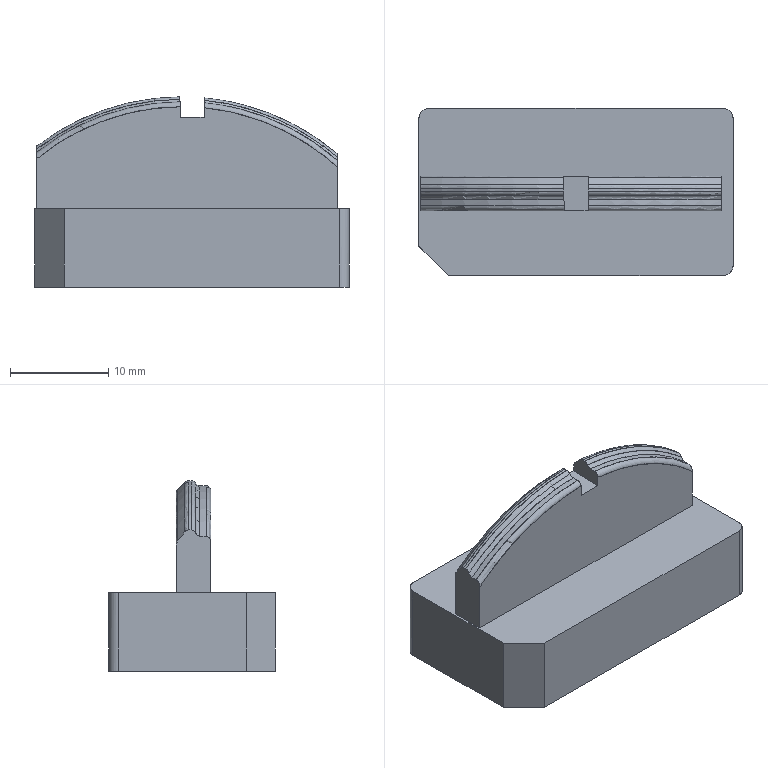NC program | PowerMill | posted with a generic post | part box 32 x 17 x 19.383 mm
Lines 7332 to 8609 of 94163:
N7429 M6
N7430 S18000 M03
N7431 G00 G90 X0.0 Y0.0
N7432 G43 Z9.8028 H28
N7433
N7434 G05 P10000 R4
N7435 X-0.7752 Y1.7566
N7436 Z0.8939
N7437 G01 Z-0.3061 F2400.0
N7438 X-0.7847 Y1.7431 F4000.0
N7439 G03 X-0.7487 Y1.5362 I0.1215 J-0.0855
N7440 G01 X-0.5198 Y1.3752
N7441 X-0.3092 Y1.0314
N7442 X-0.2501 Y0.6876
N7443 X-0.2383 Y-0.3438
N7444 X-0.3315 Y-0.6876
N7445 X-0.5157 Y-0.9547
N7446 X-0.6006 Y-1.0314
N7447 X-0.7139 Y-1.0989
N7448 X0.989 Y-1.1654
N7449 X0.993 Y-1.1494
N7450 G03 X0.8849 Y-0.9693 I-0.1441 J0.036
N7451 G01 X0.8595 Y-0.963
N7452 X0.5157 Y-0.7078
N7453 X0.3142 Y-0.3438
N7454 X0.2701 Y0.0
N7455 X0.3007 Y0.6876
N7456 X0.4429 Y1.0314
N7457 X0.5157 Y1.1263
N7458 X0.8218 Y1.3752
N7459 X0.8868 Y1.3937
N7460 X-0.732 Y1.8085 Z-0.4053
N7461 X-0.7412 Y1.7948
N7462 G03 X-0.7014 Y1.5886 I0.123 J-0.0831
N7463 G01 X-0.5157 Y1.4631
N7464 X-0.4443 Y1.3752
N7465 X-0.2825 Y1.0314
N7466 X-0.2501 Y0.6876
N7467 X-0.2324 Y-0.3438
N7468 X-0.2957 Y-0.6876
N7469 X-0.5125 Y-1.0314
N7470 X-0.6943 Y-1.1536
N7471 X0.7534 Y-1.2762
N7472 X0.7618 Y-1.262
N7473 G03 X0.7103 Y-1.0584 I-0.1275 J0.076
N7474 G01 X0.665 Y-1.0314
N7475 X0.5157 Y-0.8945
N7476 X0.3761 Y-0.6876
N7477 X0.2725 Y-0.3438
N7478 X0.2753 Y-0.0404
N7479 X0.2702 Y0.0
N7480 X0.2772 Y0.158
N7481 X0.2821 Y0.6876
N7482 X0.3501 Y1.0314
N7483 X0.5157 Y1.3119
N7484 X0.7428 Y1.4864
N7485 G00 Z3.6956
N7486 G01 X0.8139 Y-1.4168 F10000.0
N7487 G00 Z0.6956
N7488 G01 Z-0.5044 F2400.0
N7489 X0.8234 Y-1.4032 F4000.0
N7490 G03 X0.7863 Y-1.1965 I-0.1219 J0.0848
N7491 G01 X0.549 Y-1.0314
N7492 X0.3298 Y-0.6876
N7493 X0.2647 Y-0.3438
N7494 X0.2705 Y-0.0022
N7495 X0.2702 Y0.0
N7496 X0.2707 Y0.0114
N7497 X0.2821 Y0.6876
N7498 X0.317 Y1.0314
N7499 X0.4818 Y1.3752
N7500 X0.7929 Y1.6298
N7501 X-0.6948 Y1.9278
N7502 X-0.7054 Y1.9152
N7503 G03 X-0.6879 Y1.7059 I0.1134 J-0.0959
N7504 G01 X-0.5157 Y1.5603
N7505 X-0.3818 Y1.3752
N7506 X-0.2648 Y1.0314
N7507 X-0.2588 Y0.7795
N7508 X-0.2501 Y0.6876
N7509 X-0.2334 Y-0.2903
N7510 X-0.2321 Y-0.3438
N7511 X-0.2691 Y-0.6876
N7512 X-0.4459 Y-1.0314
N7513 X-0.5157 Y-1.1132
N7514 X-0.7115 Y-1.2439
N7515 G00 Z3.5964
N7516 G01 X-0.7282 Y2.0143 F10000.0
N7517 G00 Z0.5964
N7518 G01 Z-0.6036 F2400.0
N7519 X-0.7372 Y2.0005 F4000.0
N7520 G03 X-0.6939 Y1.795 I0.1244 J-0.0811
N7521 G01 X-0.5773 Y1.719
N7522 X-0.3352 Y1.3752
N7523 X-0.2568 Y1.0314
N7524 X-0.2547 Y0.7352
N7525 X-0.2502 Y0.6876
N7526 X-0.2335 Y-0.2903
N7527 X-0.2448 Y-0.4888
N7528 X-0.2444 Y-0.6876
N7529 X-0.3743 Y-1.0314
N7530 X-0.5157 Y-1.2143
N7531 X-0.6781 Y-1.3402
N7532 X0.8326 Y-1.5085
N7533 X0.8423 Y-1.4951
N7534 G03 X0.8096 Y-1.2877 I-0.1201 J0.0874
N7535 G01 X0.5157 Y-1.0737
N7536 X0.3028 Y-0.6876
N7537 X0.2641 Y-0.3438
N7538 X0.2661 Y-0.265
N7539 X0.2774 Y0.3833
N7540 X0.2987 Y1.0314
N7541 X0.4188 Y1.3752
N7542 X0.5157 Y1.5155
N7543 X0.7468 Y1.719
N7544 X0.7836 Y1.7396
N7545 X-0.7258 Y2.1271 Z-0.7027
N7546 X-0.7355 Y2.1136
N7547 G03 X-0.7014 Y1.9064 I0.1207 J-0.0865
N7548 G01 X-0.5157 Y1.7731
N7549 X-0.2954 Y1.3752
N7550 X-0.2561 Y1.0314
N7551 X-0.2141 Y-1.3752
N7552 X-0.2196 Y-1.5267
N7553 X0.7835 Y-1.597
N7554 X0.7914 Y-1.5826
N7555 G03 X0.7325 Y-1.381 I-0.1302 J0.0714
N7556 G01 X0.722 Y-1.3752
N7557 X0.5157 Y-1.2015
N7558 X0.3934 Y-1.0314
N7559 X0.2727 Y-0.6876
N7560 X0.275 Y-0.4396
N7561 X0.2646 Y-0.3526
N7562 X0.2661 Y-0.265
N7563 X0.2706 Y-0.0022
N7564 X0.2703 Y0.0
N7565 X0.2708 Y0.0114
N7566 X0.2822 Y0.6876
N7567 X0.2854 Y0.719
N7568 X0.2882 Y1.0314
N7569 X0.3629 Y1.3752
N7570 X0.5157 Y1.6302
N7571 X0.5999 Y1.719
N7572 X0.7719 Y1.8377
N7573 G00 Z3.3981
N7574 G01 X0.1689 Y-2.2838 F10000.0
N7575 G00 Z0.3981
N7576 G01 Z-0.8019 F2400.0
N7577 X0.1949 Y-2.2744 F4000.0
N7578 G03 X0.344 Y-1.9554 I-0.085 J0.234
N7579 G01 X0.2581 Y-1.719
N7580 X0.2461 Y-1.3752
N7581 X0.2881 Y1.0314
N7582 X0.3287 Y1.3752
N7583 X0.5055 Y1.719
N7584 X0.7943 Y1.9494
N7585 X-0.6914 Y2.2352
N7586 X-0.7019 Y2.2224
N7587 G03 X-0.6821 Y2.0134 I0.1144 J-0.0946
N7588 G01 X-0.5157 Y1.8759
N7589 X-0.401 Y1.719
N7590 X-0.2746 Y1.3752
N7591 X-0.2561 Y1.0314
N7592 X-0.2081 Y-1.719
N7593 X-0.2573 Y-2.0628
N7594 X-0.3481 Y-2.2225
N7595 G00 Z3.299
N7596 G01 X-0.7622 Y2.332 F10000.0
N7597 G00 Z0.299
N7598 G01 Z-0.901 F2400.0
N7599 X-0.7708 Y2.3179 F4000.0
N7600 G03 X-0.7211 Y2.1138 I0.1269 J-0.0773
N7601 G01 X-0.6373 Y2.0628
N7602 X-0.5157 Y1.9492
N7603 X-0.3619 Y1.719
N7604 X-0.2657 Y1.3752
N7605 X-0.2561 Y1.0314
N7606 X-0.2081 Y-1.719
N7607 X-0.2362 Y-2.0628
N7608 X-0.3945 Y-2.4066
N7609 X-0.5157 Y-2.5454
N7610 X-0.6865 Y-2.6561
N7611 X0.7717 Y-2.7798
N7612 X0.781 Y-2.7661
N7613 G03 X0.7417 Y-2.5598 I-0.1228 J0.0835
N7614 G01 X0.5164 Y-2.4066
N7615 X0.3027 Y-2.0628
N7616 X0.2403 Y-1.719
N7617 X0.2462 Y-1.3801
N7618 Y-1.3776
N7619 Y-1.3752
N7620 X0.2752 Y0.2892
N7621 X0.2881 Y1.0314
N7622 X0.3122 Y1.3752
N7623 X0.4536 Y1.719
N7624 X0.5157 Y1.8048
N7625 X0.8141 Y2.044
N7626 X-0.7429 Y2.4159 Z-1.0002
N7627 X-0.7525 Y2.4025
N7628 G03 X-0.7177 Y2.1954 I0.1209 J-0.0862
N7629 G01 X-0.5317 Y2.0628
N7630 X-0.3213 Y1.719
N7631 X-0.262 Y1.3752
N7632 X-0.2081 Y-1.719
N7633 X-0.2222 Y-2.0628
N7634 X-0.3527 Y-2.4066
N7635 X-0.5157 Y-2.6085
N7636 X-0.6882 Y-2.7374
N7637 X0.7995 Y-2.8968
N7638 X0.8086 Y-2.8831
N7639 G03 X0.7671 Y-2.6772 I-0.1237 J0.0822
N7640 G01 X0.5157 Y-2.5102
N7641 X0.4302 Y-2.4066
N7642 X0.269 Y-2.0628
N7643 X0.24 Y-1.719
N7644 X0.2881 Y1.0314
N7645 X0.2989 Y1.3752
N7646 X0.3985 Y1.719
N7647 X0.5157 Y1.9012
N7648 X0.6829 Y2.0628
N7649 X0.7869 Y2.1276
N7650 X-0.7503 Y2.5005 Z-1.0993
N7651 X-0.7597 Y2.4869
N7652 G03 X-0.722 Y2.2803 I0.1221 J-0.0845
N7653 G01 X-0.5157 Y2.1375
N7654 X-0.456 Y2.0628
N7655 X-0.2947 Y1.719
N7656 X-0.262 Y1.3752
N7657 X-0.2081 Y-1.719
N7658 X-0.2158 Y-2.0628
N7659 X-0.3327 Y-2.4066
N7660 X-0.5157 Y-2.6418
N7661 X-0.6538 Y-2.7504
N7662 X-0.748 Y-2.7974
N7663 X0.8439 Y-2.9825
N7664 X0.8512 Y-2.9676
N7665 G03 X0.7829 Y-2.769 I-0.1335 J0.0651
N7666 G01 X0.7447 Y-2.7504
N7667 X0.5157 Y-2.572
N7668 X0.3874 Y-2.4066
N7669 X0.2551 Y-2.0628
N7670 X0.24 Y-1.719
N7671 X0.2941 Y1.3752
N7672 X0.3576 Y1.719
N7673 X0.5157 Y1.9977
N7674 X0.7992 Y2.2227
N7675 X-0.7467 Y2.6019 Z-1.1985
N7676 X-0.7572 Y2.5891
N7677 G03 X-0.7356 Y2.3802 I0.1153 J-0.0937
N7678 G01 X-0.5157 Y2.2014
N7679 X-0.4132 Y2.0628
N7680 X-0.2814 Y1.719
N7681 X-0.262 Y1.3752
N7682 X-0.2081 Y-1.719
N7683 X-0.2135 Y-2.0628
N7684 X-0.326 Y-2.4066
N7685 X-0.5157 Y-2.6539
N7686 X-0.6342 Y-2.7504
N7687 X-0.766 Y-2.8189
N7688 X0.8581 Y-3.0262
N7689 X0.8657 Y-3.0116
N7690 G03 X0.803 Y-2.8112 I-0.1316 J0.0689
N7691 G01 X0.6868 Y-2.7504
N7692 X0.5157 Y-2.6079
N7693 X0.3688 Y-2.4066
N7694 X0.2485 Y-2.0628
N7695 X0.24 Y-1.719
N7696 X0.2941 Y1.3752
N7697 X0.3297 Y1.719
N7698 X0.495 Y2.0628
N7699 X0.8074 Y2.321
N7700 X-0.8243 Y2.6593 Z-1.2976
N7701 X-0.8323 Y2.6449
N7702 G03 X-0.7743 Y2.4431 I0.1299 J-0.0719
N7703 G01 X-0.7084 Y2.4066
N7704 X-0.5157 Y2.2373
N7705 X-0.3919 Y2.0628
N7706 X-0.2777 Y1.719
N7707 X-0.262 Y1.3752
N7708 X-0.2081 Y-1.719
N7709 X-0.2134 Y-2.0628
N7710 X-0.3256 Y-2.4066
N7711 X-0.5157 Y-2.6545
N7712 X-0.6333 Y-2.7504
N7713 X-0.7717 Y-2.8224
N7714 X0.8512 Y-3.0375
N7715 X0.859 Y-3.023
N7716 G03 X0.7991 Y-2.8217 I-0.1306 J0.0707
N7717 G01 X0.6673 Y-2.7504
N7718 X0.5157 Y-2.6213
N7719 X0.3584 Y-2.4066
N7720 X0.2457 Y-2.0628
N7721 X0.24 Y-1.719
N7722 X0.2941 Y1.3752
N7723 X0.3153 Y1.719
N7724 X0.4495 Y2.0628
N7725 X0.5157 Y2.1557
N7726 X0.808 Y2.4026
N7727 X-0.8191 Y2.6665 Z-1.3968
N7728 X-0.827 Y2.652
N7729 G03 X-0.7675 Y2.4506 I0.1305 J-0.0709
N7730 G01 X-0.6864 Y2.4066
N7731 X-0.5157 Y2.251
N7732 X-0.3838 Y2.0628
N7733 X-0.2743 Y1.719
N7734 X-0.262 Y1.3752
N7735 X-0.2081 Y-1.719
N7736 X-0.2134 Y-2.0628
N7737 X-0.3256 Y-2.4066
N7738 X-0.5157 Y-2.6545
N7739 X-0.6333 Y-2.7504
N7740 X-0.7725 Y-2.8229
N7741 X0.8509 Y-3.0387
N7742 X0.8588 Y-3.0242
N7743 G03 X0.799 Y-2.8229 I-0.1306 J0.0707
N7744 G01 X0.6653 Y-2.7504
N7745 X0.5157 Y-2.6227
N7746 X0.3576 Y-2.4066
N7747 X0.2455 Y-2.0628
N7748 X0.24 Y-1.719
N7749 X0.2941 Y1.3752
N7750 X0.3091 Y1.719
N7751 X0.4275 Y2.0628
N7752 X0.5157 Y2.1958
N7753 X0.7473 Y2.4066
N7754 X0.8096 Y2.4425
N7755 X-0.8267 Y2.672 Z-1.4959
N7756 X-0.8346 Y2.6575
N7757 G03 X-0.7745 Y2.4562 I0.1307 J-0.0706
N7758 G01 X-0.6827 Y2.4066
N7759 X-0.5157 Y2.2525
N7760 X-0.3826 Y2.0628
N7761 X-0.2739 Y1.719
N7762 X-0.262 Y1.3752
N7763 X-0.2081 Y-1.719
N7764 X-0.2134 Y-2.0628
N7765 X-0.3256 Y-2.4066
N7766 X-0.5157 Y-2.6546
N7767 X-0.6333 Y-2.7504
N7768 X-0.7725 Y-2.8229
N7769 X0.8509 Y-3.0388
N7770 X0.8588 Y-3.0242
N7771 G03 X0.799 Y-2.8229 I-0.1306 J0.0707
N7772 G01 X0.6653 Y-2.7504
N7773 X0.5157 Y-2.6227
N7774 X0.3576 Y-2.4066
N7775 X0.2455 Y-2.0628
N7776 X0.24 Y-1.719
N7777 X0.2941 Y1.3752
N7778 X0.3063 Y1.719
N7779 X0.4166 Y2.0628
N7780 X0.5157 Y2.2115
N7781 X0.7202 Y2.4066
N7782 X0.8053 Y2.4569
N7783 X-0.8264 Y2.6737 Z-1.5951
N7784 X-0.8343 Y2.6592
N7785 G03 X-0.7756 Y2.4576 I0.1302 J-0.0714
N7786 G01 X-0.6827 Y2.4066
N7787 X-0.5157 Y2.2541
N7788 X-0.3826 Y2.0628
N7789 X-0.2739 Y1.719
N7790 X-0.262 Y1.3752
N7791 X-0.2081 Y-1.719
N7792 X-0.2134 Y-2.0628
N7793 X-0.3256 Y-2.4066
N7794 X-0.5157 Y-2.6546
N7795 X-0.6333 Y-2.7504
N7796 X-0.7725 Y-2.8229
N7797 X0.8509 Y-3.0388
N7798 X0.8587 Y-3.0243
N7799 G03 X0.799 Y-2.8229 I-0.1305 J0.0708
N7800 G01 X0.6652 Y-2.7504
N7801 X0.5157 Y-2.6227
N7802 X0.3576 Y-2.4066
N7803 X0.2455 Y-2.0628
N7804 X0.24 Y-1.719
N7805 X0.2941 Y1.3752
N7806 X0.3058 Y1.719
N7807 X0.4145 Y2.0628
N7808 X0.5157 Y2.2133
N7809 X0.7146 Y2.4066
N7810 X0.8055 Y2.4591
N7811 X-0.8247 Y2.6747 Z-1.6942
N7812 X-0.8328 Y2.6603
N7813 G03 X-0.7753 Y2.4583 I0.1298 J-0.0723
N7814 G01 X-0.6826 Y2.4066
N7815 X-0.5157 Y2.2557
N7816 X-0.3826 Y2.0628
N7817 X-0.2738 Y1.719
N7818 X-0.262 Y1.3752
N7819 X-0.2081 Y-1.719
N7820 X-0.2134 Y-2.0628
N7821 X-0.3256 Y-2.4066
N7822 X-0.5157 Y-2.6546
N7823 X-0.6332 Y-2.7504
N7824 X-0.7725 Y-2.8229
N7825 X0.8509 Y-3.0388
N7826 X0.8587 Y-3.0243
N7827 G03 X0.799 Y-2.8229 I-0.1305 J0.0708
N7828 G01 X0.6652 Y-2.7504
N7829 X0.5157 Y-2.6228
N7830 X0.3576 Y-2.4066
N7831 X0.2454 Y-2.0628
N7832 X0.24 Y-1.719
N7833 X0.2941 Y1.3752
N7834 X0.3058 Y1.719
N7835 X0.4145 Y2.0628
N7836 X0.5157 Y2.2151
N7837 X0.7146 Y2.4066
N7838 X0.8052 Y2.4598
N7839 X-0.8231 Y2.6757 Z-1.7934
N7840 X-0.8312 Y2.6613
N7841 G03 X-0.7751 Y2.4589 I0.1292 J-0.0731
N7842 G01 X-0.6826 Y2.4066
N7843 X-0.5157 Y2.2572
N7844 X-0.3826 Y2.0628
N7845 X-0.2738 Y1.719
N7846 X-0.262 Y1.3752
N7847 X-0.2081 Y-1.719
N7848 X-0.2134 Y-2.0628
N7849 X-0.3256 Y-2.4066
N7850 X-0.5157 Y-2.6546
N7851 X-0.6332 Y-2.7504
N7852 X-0.7725 Y-2.8229
N7853 X0.8508 Y-3.0388
N7854 X0.8587 Y-3.0243
N7855 G03 X0.799 Y-2.8229 I-0.1305 J0.0708
N7856 G01 X0.6652 Y-2.7504
N7857 X0.5157 Y-2.6228
N7858 X0.3576 Y-2.4066
N7859 X0.2454 Y-2.0628
N7860 X0.24 Y-1.719
N7861 X0.2941 Y1.3752
N7862 X0.3058 Y1.719
N7863 X0.4145 Y2.0628
N7864 X0.5157 Y2.2169
N7865 X0.7146 Y2.4066
N7866 X0.8048 Y2.4604
N7867 X-0.8215 Y2.6766 Z-1.8925
N7868 X-0.8297 Y2.6623
N7869 G03 X-0.7749 Y2.4596 I0.1288 J-0.0739
N7870 G01 X-0.6826 Y2.4066
N7871 X-0.5157 Y2.2588
N7872 X-0.3825 Y2.0628
N7873 X-0.2738 Y1.719
N7874 X-0.262 Y1.3752
N7875 X-0.208 Y-1.719
N7876 X-0.2133 Y-2.0628
N7877 X-0.3256 Y-2.4066
N7878 X-0.5157 Y-2.6546
N7879 X-0.6332 Y-2.7504
N7880 X-0.7724 Y-2.8229
N7881 X0.8508 Y-3.0388
N7882 X0.8587 Y-3.0243
N7883 G03 X0.799 Y-2.8229 I-0.1305 J0.0708
N7884 G01 X0.6652 Y-2.7504
N7885 X0.5157 Y-2.6228
N7886 X0.3575 Y-2.4066
N7887 X0.2454 Y-2.0628
N7888 X0.24 Y-1.719
N7889 X0.294 Y1.3752
N7890 X0.3058 Y1.719
N7891 X0.4145 Y2.0628
N7892 X0.5157 Y2.2187
N7893 X0.7146 Y2.4066
N7894 X0.8045 Y2.4611
N7895 X-0.8199 Y2.6776 Z-1.9917
N7896 X-0.8283 Y2.6634
N7897 G03 X-0.7747 Y2.4603 I0.1283 J-0.0748
N7898 G01 X-0.6826 Y2.4066
N7899 X-0.5157 Y2.2603
N7900 X-0.3825 Y2.0628
N7901 X-0.2738 Y1.719
N7902 X-0.262 Y1.3752
N7903 X-0.208 Y-1.719
N7904 X-0.2133 Y-2.0628
N7905 X-0.3256 Y-2.4066
N7906 X-0.5157 Y-2.6546
N7907 X-0.6332 Y-2.7504
N7908 X-0.7724 Y-2.8229
N7909 X0.8508 Y-3.0388
N7910 X0.8587 Y-3.0243
N7911 G03 X0.7989 Y-2.8229 I-0.1306 J0.0708
N7912 G01 X0.6652 Y-2.7504
N7913 X0.5157 Y-2.6228
N7914 X0.3575 Y-2.4066
N7915 X0.2454 Y-2.0628
N7916 X0.24 Y-1.719
N7917 X0.294 Y1.3752
N7918 X0.3058 Y1.719
N7919 X0.4145 Y2.0628
N7920 X0.5157 Y2.2205
N7921 X0.7146 Y2.4066
N7922 X0.8043 Y2.4618
N7923 X-0.8184 Y2.6786 Z-2.0908
N7924 X-0.8268 Y2.6644
N7925 G03 X-0.7745 Y2.4609 I0.1279 J-0.0756
N7926 G01 X-0.6826 Y2.4066
N7927 X-0.5157 Y2.2619
N7928 X-0.3825 Y2.0628
N7929 X-0.2738 Y1.719
N7930 X-0.262 Y1.3752
N7931 X-0.208 Y-1.719
N7932 X-0.2133 Y-2.0628
N7933 X-0.3256 Y-2.4066
N7934 X-0.5157 Y-2.6546
N7935 X-0.6332 Y-2.7504
N7936 X-0.7724 Y-2.8229
N7937 X0.8508 Y-3.0388
N7938 X0.8587 Y-3.0243
N7939 G03 X0.7989 Y-2.8229 I-0.1306 J0.0708
N7940 G01 X0.6652 Y-2.7504
N7941 X0.5157 Y-2.6228
N7942 X0.3575 Y-2.4066
N7943 X0.2454 Y-2.0628
N7944 X0.24 Y-1.719
N7945 X0.294 Y1.3752
N7946 X0.3057 Y1.719
N7947 X0.4145 Y2.0628
N7948 X0.5157 Y2.2223
N7949 X0.7146 Y2.4066
N7950 X0.804 Y2.4625
N7951 X-0.8168 Y2.6795 Z-2.19
N7952 X-0.8253 Y2.6653
N7953 G03 X-0.7743 Y2.4616 I0.1274 J-0.0764
N7954 G01 X-0.6826 Y2.4066
N7955 X-0.5157 Y2.2635
N7956 X-0.3825 Y2.0628
N7957 X-0.2738 Y1.719
N7958 X-0.2619 Y1.3752
N7959 X-0.208 Y-1.719
N7960 X-0.2133 Y-2.0628
N7961 X-0.3256 Y-2.4066
N7962 X-0.5157 Y-2.6546
N7963 X-0.6332 Y-2.7504
N7964 X-0.7724 Y-2.8229
N7965 X0.8508 Y-3.0388
N7966 X0.8586 Y-3.0243
N7967 G03 X0.7989 Y-2.8229 I-0.1305 J0.0708
N7968 G01 X0.6652 Y-2.7504
N7969 X0.5157 Y-2.6228
N7970 X0.3575 Y-2.4066
N7971 X0.2454 Y-2.0628
N7972 X0.24 Y-1.719
N7973 X0.294 Y1.3752
N7974 X0.3057 Y1.719
N7975 X0.4145 Y2.0628
N7976 X0.5157 Y2.2241
N7977 X0.7145 Y2.4066
N7978 X0.8037 Y2.4631
N7979 G00 Z2.932
N7980 G01 X0.8508 Y-3.0388 F10000.0
N7981 G00 Z-1.0891
N7982 G01 Z-2.2891 F2400.0
N7983 X0.8586 Y-3.0243 F4000.0
N7984 G03 X0.7989 Y-2.8229 I-0.1305 J0.0708
N7985 G01 X0.6652 Y-2.7504
N7986 X0.5157 Y-2.6228
N7987 X0.3575 Y-2.4066
N7988 X0.2454 Y-2.0628
N7989 Y-2.0605
N7990 X0.24 Y-1.719
N7991 X0.2623 Y-0.4423
N7992 X0.2301 Y-0.3781
N7993 X0.1631 Y-0.3521
N7994 X-0.1292 Y-0.3512
N7995 G03 X-0.2295 Y-0.4529 I-0.0003 J-0.1
N7996 G01 X-0.208 Y-1.719
N7997 X-0.2133 Y-2.0628
N7998 X-0.3255 Y-2.4066
N7999 X-0.5157 Y-2.6546
N8000 X-0.6332 Y-2.7504
N8001 X-0.7724 Y-2.8229
N8002 G00 Z9.8028
N8003 G05 P0
N8004 (---------------)
N8005 ( END TOOLPATH : 精公再粗03-外形偏置-D2C )
N8006 (---------------)
N8007
N8008 M05
N8009 G53 Z0.0
N8010 (---------------)
N8011 ( START TOOLPATH : 精公基准台01-基准面偏置-D10 )
N8012 (---------------)
N8013 ( TOOL NO.    :3 )
N8014 ( TOOL TYPE   : ENDMILL)
N8015 ( TOOL ID     : D10_1_1_1)
N8016 ( TOOL DIA    : 10.0 LENGTH 74.56)
N8017 T3
N8018 M6
N8019 S8500 M03
N8020 G00 G90 X0.0 Y0.0
N8021 G43 Z9.8028 H3
N8022
N8023 G05 P10000 R8
N8024 X24.6171 Y14.2541
N8025 Z-10.38
N8026 G01 Z-11.58 F360.0
N8027 X20.326 Y11.1862 F600.0
N8028 X11.9023 Y6.9744
N8029 X14.8097
N8030 X15.0912 Y6.967
N8031 X15.372 Y6.9449
N8032 X15.6513 Y6.9082
N8033 X15.9282 Y6.8568
N8034 X16.2021 Y6.7911
N8035 X16.4722 Y6.7111
N8036 X16.7377 Y6.6171
N8037 X16.9979 Y6.5093
N8038 X17.2521 Y6.388
N8039 X17.4997 Y6.2536
N8040 X17.7398 Y6.1065
N8041 X17.972 Y5.9469
N8042 G02 X18.4096 Y5.5925 I-3.8476 J-5.1989
N8043 G02 X18.8078 Y5.1943 I-4.183 J-4.581
N8044 G01 X19.0341 Y4.9236
N8045 X19.1622 Y4.7567
N8046 X19.3217 Y4.5246
N8047 X19.4689 Y4.2844
N8048 X19.6033 Y4.0369
N8049 X19.7245 Y3.7827
N8050 X19.8323 Y3.5224
N8051 X19.9264 Y3.2569
N8052 X20.0063 Y2.9868
N8053 X20.0721 Y2.713
N8054 X20.1234 Y2.436
N8055 X20.1602 Y2.1568
N8056 X20.1823 Y1.876
N8057 X20.1897 Y1.5944
N8058 Y-1.9296
N8059 X20.1823 Y-2.2112
N8060 X20.1602 Y-2.492
N8061 X20.1234 Y-2.7712
N8062 X20.0721 Y-3.0482
N8063 X20.0064 Y-3.322
N8064 G02 X19.8323 Y-3.8576 I-6.0957 J1.6847
N8065 G01 X19.7245 Y-4.1178
N8066 X19.6033 Y-4.3721
N8067 X19.4689 Y-4.6196
N8068 X19.3217 Y-4.8598
N8069 X19.1622 Y-5.0919
N8070 X18.9907 Y-5.3153
N8071 X18.8078 Y-5.5295
N8072 G02 X18.4096 Y-5.9277 I-4.5588 J4.1606
N8073 G01 X18.1954 Y-6.1106
N8074 X17.972 Y-6.2821
N8075 X17.7398 Y-6.4416
N8076 X17.4997 Y-6.5888
N8077 X17.2521 Y-6.7232
N8078 X16.9979 Y-6.8445
N8079 X16.7377 Y-6.9523
N8080 X16.4722 Y-7.0463
N8081 X16.2021 Y-7.1263
N8082 X15.9282 Y-7.192
N8083 X15.6513 Y-7.2434
N8084 X15.372 Y-7.2801
N8085 X15.0912 Y-7.3022
N8086 X14.8097 Y-7.3096
N8087 X-15.7937
N8088 X-16.0752 Y-7.3022
N8089 X-16.356 Y-7.2801
N8090 X-16.6353 Y-7.2434
N8091 X-16.9122 Y-7.192
N8092 X-17.1861 Y-7.1263
N8093 X-17.4562 Y-7.0463
N8094 X-17.7217 Y-6.9523
N8095 X-17.9819 Y-6.8445
N8096 X-18.2361 Y-6.7232
N8097 X-18.4837 Y-6.5888
N8098 X-18.7238 Y-6.4416
N8099 X-18.956 Y-6.2821
N8100 X-19.1794 Y-6.1106
N8101 X-19.3936 Y-5.9277
N8102 X-19.5979 Y-5.7338
N8103 X-19.7918 Y-5.5295
N8104 X-19.9747 Y-5.3153
N8105 X-20.1462 Y-5.0919
N8106 X-20.3057 Y-4.8598
N8107 X-20.4529 Y-4.6196
N8108 X-20.5873 Y-4.3721
N8109 X-20.7085 Y-4.1178
N8110 X-20.8163 Y-3.8576
N8111 X-20.9103 Y-3.5921
N8112 X-20.9903 Y-3.322
N8113 X-21.0561 Y-3.0482
N8114 X-21.1074 Y-2.7712
N8115 X-21.1442 Y-2.492
N8116 X-21.1663 Y-2.2112
N8117 X-21.1737 Y-1.9296
N8118 Y1.5944
N8119 X-21.1663 Y1.876
N8120 X-21.1442 Y2.1568
N8121 X-21.1169 Y2.3641
N8122 X-21.089 Y2.539
N8123 X-21.0561 Y2.713
N8124 X-20.9904 Y2.9868
N8125 X-20.9103 Y3.2569
N8126 X-20.8163 Y3.5224
N8127 X-20.7085 Y3.7826
N8128 X-20.5873 Y4.0369
N8129 X-20.4529 Y4.2844
N8130 X-20.3057 Y4.5246
N8131 X-20.1462 Y4.7567
N8132 X-19.9747 Y4.9801
N8133 X-19.7918 Y5.1943
N8134 X-19.5979 Y5.3986
N8135 X-19.3936 Y5.5925
N8136 X-19.1794 Y5.7754
N8137 X-18.9559 Y5.9469
N8138 X-18.7238 Y6.1064
N8139 X-18.4837 Y6.2536
N8140 X-18.2361 Y6.388
N8141 X-17.9819 Y6.5093
N8142 X-17.7217 Y6.6171
N8143 X-17.4562 Y6.7111
N8144 X-17.1861 Y6.7911
N8145 X-16.9122 Y6.8568
N8146 X-16.6353 Y6.9082
N8147 X-16.356 Y6.9449
N8148 X-16.0752 Y6.967
N8149 X-15.7937 Y6.9744
N8150 X11.9023
N8151 G00 Z9.8028
N8152 G05 P0
N8153 (---------------)
N8154 ( END TOOLPATH : 精公基准台01-基准面偏置-D10 )
N8155 (---------------)
N8156 ( START TOOLPATH : 精公基准台01-外形侧光-D10 )
N8157 (---------------)
N8158 G00 X0.0 Y0.0 Z10.803
N8159 G05 P10000 R8
N8160 X18.0226 Y-6.4569
N8161 Z-10.35
N8162 G01 Z-11.55 F360.0
N8163 G03 X16.8752 Y-6.494 I-0.5289 J-1.4036 F600.0
N8164 G02 X14.7871 Y-6.9396 I-2.0657 J4.5645
N8165 G01 X-0.4564 Y-6.9392
N8166 X-15.8853 Y-6.9388
N8167 G02 X-20.803 Y-2.0081 I0.0916 J5.0092
N8168 G01 X-20.8034 Y1.6453
N8169 G02 X-15.8824 Y6.6036 I5.0097 J-0.0509
N8170 G01 X5.2011 Y6.6041
N8171 X14.7882 Y6.6044
N8172 G02 X19.8194 Y1.643 I0.0213 J-5.0102
N8173 G01 X19.819 Y-2.0109
N8174 G02 X16.8752 Y-6.494 I-5.0095 J0.0814
N8175 G03 X16.09 Y-7.3315 I0.6185 J-1.3665
N8176 G01 X17.9163 Y-6.4355
N8177 G03 X16.7684 Y-6.4538 I-0.552 J-1.3948
N8178 G02 X14.7871 Y-6.8596 I-1.9589 J4.5243
N8179 G01 X-0.4564
N8180 X-15.6998
N8181 G02 X-20.723 Y-2.0081 I-0.0911 J4.932
N8182 G01 X-20.7234 Y1.643
N8183 G02 X-15.6998 Y6.5244 I4.9325 J-0.0505
N8184 G01 X5.2011
N8185 X14.7871
N8186 G02 X19.7394 Y1.643 I0.0224 J-4.9301
N8187 G01 X19.739 Y-2.0081
N8188 G02 X16.7684 Y-6.4538 I-4.9295 J0.0786
N8189 G03 X15.9696 Y-7.2784 I0.596 J-1.3765
N8190 G00 Z10.803
N8191 G05 P0
N8192 (---------------)
N8193 ( END TOOLPATH : 精公基准台01-外形侧光-D10 )
N8194 (---------------)
N8195 ( START TOOLPATH : 精公基准台01-基准台侧光-D10 )
N8196 (---------------)
N8197 G00 X0.0 Y0.0 Z9.8028
N8198 G05 P10000 R8
N8199 X21.3365 Y-16.5868
N8200 Z-18.28
N8201 G01 Z-19.48 F360.0
N8202 G03 X18.475 Y-12.4866 I-1.4307 J2.0501 F600.0
N8203 G01 X18.3822 Y-12.5513
N8204 X18.3809 Y-12.5523
N8205 X18.3795 Y-12.5532
N8206 X18.1285 Y-12.7133
N8207 X18.1263 Y-12.7146
N8208 X18.1241 Y-12.7159
N8209 X17.7428 Y-12.9261
N8210 X17.7405 Y-12.9273
N8211 X17.7381 Y-12.9285
N8212 X17.422 Y-13.0767
N8213 X17.4199 Y-13.0776
N8214 X17.4178 Y-13.0785
N8215 X17.1016 Y-13.2052
N8216 X17.0995 Y-13.206
N8217 X17.0974 Y-13.2068
N8218 X16.7812 Y-13.3131
N8219 X16.7797 Y-13.3136
N8220 X16.7782 Y-13.3141
N8221 X16.6388 Y-13.3549
N8222 X16.6377 Y-13.3552
N8223 X16.6367 Y-13.3555
N8224 X16.4599 Y-13.402
N8225 X16.4583 Y-13.4024
N8226 X16.4566 Y-13.4028
N8227 X16.1405 Y-13.4718
N8228 X16.1384 Y-13.4722
N8229 X16.1364 Y-13.4726
N8230 X15.8202 Y-13.5244
N8231 X15.8181 Y-13.5247
N8232 X15.8159 Y-13.525
N8233 X15.4997 Y-13.5591
N8234 X15.4976 Y-13.5593
N8235 X15.4955 Y-13.5595
N8236 X15.1794 Y-13.5768
N8237 X15.1776 Y-13.5769
N8238 X15.1758
N8239 X14.8596 Y-13.58
N8240 X14.8592
N8241 X14.8588
N8242 X-12.962
N8243 X-12.963
N8244 X-12.9639
N8245 X-13.2801 Y-13.5722
N8246 X-13.2826 Y-13.5721
N8247 X-13.2851 Y-13.572
N8248 X-13.6012 Y-13.5443
N8249 X-13.6038 Y-13.544
N8250 X-13.6063 Y-13.5437
N8251 X-13.9225 Y-13.4955
N8252 X-13.925 Y-13.4951
N8253 X-13.9275 Y-13.4946
N8254 X-14.2437 Y-13.4254
N8255 X-14.2459 Y-13.4249
N8256 X-14.2482 Y-13.4243
N8257 X-14.4946 Y-13.3551
N8258 X-14.4971 Y-13.3544
N8259 X-14.4996 Y-13.3535
N8260 X-14.8855 Y-13.2171
N8261 X-14.8884 Y-13.216
N8262 X-14.8911 Y-13.2148
N8263 X-15.2073 Y-13.0754
N8264 X-15.2098 Y-13.0742
N8265 X-15.2123 Y-13.0729
N8266 X-15.5285 Y-12.906
N8267 X-15.531 Y-12.9046
N8268 X-15.5335 Y-12.9031
N8269 X-15.8374 Y-12.7137
N8270 X-15.8399 Y-12.712
N8271 X-15.8424 Y-12.7103
N8272 X-16.1708 Y-12.4689
N8273 X-16.1725 Y-12.4676
N8274 X-16.1741 Y-12.4663
N8275 X-16.2653 Y-12.3916
N8276 X-16.2666 Y-12.3905
N8277 X-16.2678 Y-12.3894
N8278 X-16.4928 Y-12.1887
N8279 X-16.4942 Y-12.1874
N8280 X-16.4955 Y-12.1861
N8281 X-16.6135 Y-12.0707
N8282 X-16.6138 Y-12.0704
N8283 X-16.6141 Y-12.0701
N8284 X-19.6576 Y-9.0254
N8285 X-19.6586 Y-9.0244
N8286 X-19.6595 Y-9.0234
N8287 X-19.7684 Y-8.9067
N8288 X-19.7697 Y-8.9052
N8289 X-19.771 Y-8.9038
N8290 X-19.9782 Y-8.6591
N8291 X-19.9793 Y-8.6578
N8292 X-19.9803 Y-8.6565
N8293 X-20.0359 Y-8.5851
N8294 X-20.0371 Y-8.5836
N8295 X-20.0382 Y-8.582
N8296 X-20.261 Y-8.2659
N8297 X-20.2627 Y-8.2634
N8298 X-20.2643 Y-8.2608
N8299 X-20.453 Y-7.9447
N8300 X-20.4545 Y-7.9421
N8301 X-20.4558 Y-7.9396
N8302 X-20.6149 Y-7.6234
N8303 X-20.6161 Y-7.6209
N8304 X-20.6172 Y-7.6184
N8305 X-20.7495 Y-7.3022
N8306 X-20.7505 Y-7.2997
N8307 X-20.7514 Y-7.2972
N8308 X-20.8593 Y-6.981
N8309 X-20.8601 Y-6.9786
N8310 X-20.8608 Y-6.9761
N8311 X-20.9428 Y-6.6723
N8312 X-20.9435 Y-6.6698
N8313 X-20.944 Y-6.6673
N8314 X-21.0103 Y-6.3387
N8315 X-21.0107 Y-6.3361
N8316 X-21.0111 Y-6.3336
N8317 X-21.0535 Y-6.0174
N8318 X-21.0538 Y-6.0149
N8319 X-21.0541 Y-6.0124
N8320 X-21.0762 Y-5.6962
N8321 X-21.0763 Y-5.6939
N8322 X-21.0764 Y-5.6915
N8323 X-21.08 Y-5.3754
N8324 Y-5.3749
N8325 Y-5.3745
N8326 X-21.0792 Y7.5875
N8327 Y7.5891
N8328 Y7.5907
N8329 X-21.0664 Y7.9069
N8330 X-21.0662 Y7.909
N8331 X-21.0661 Y7.9112
N8332 X-21.0363 Y8.2273
N8333 X-21.036 Y8.2294
N8334 X-21.0358 Y8.2315
N8335 X-20.989 Y8.5476
N8336 X-20.9887 Y8.5494
N8337 X-20.9884 Y8.5513
N8338 X-20.9441 Y8.7781
N8339 X-20.9437 Y8.7802
N8340 X-20.9432 Y8.7823
N8341 X-20.8409 Y9.1878
N8342 X-20.8402 Y9.1902
N8343 X-20.8395 Y9.1926
N8344 X-20.7384 Y9.5087
N8345 X-20.7377 Y9.5108
N8346 X-20.737 Y9.5128
N8347 X-20.6243 Y9.8095
N8348 X-20.6234 Y9.8117
N8349 X-20.6225 Y9.8138
N8350 X-20.4722 Y10.1494
N8351 X-20.4712 Y10.1515
N8352 X-20.4701 Y10.1537
N8353 X-20.3052 Y10.4698
N8354 X-20.304 Y10.4719
N8355 X-20.3028 Y10.4741
N8356 X-20.1126 Y10.7902
N8357 X-20.1116 Y10.7919
N8358 X-20.1105 Y10.7935
N8359 X-19.9836 Y10.9828
N8360 X-19.9829 Y10.9839
N8361 X-19.9821 Y10.9849
N8362 X-19.8909 Y11.1118
N8363 X-19.8899 Y11.1132
N8364 X-19.8888 Y11.1146
N8365 X-19.6639 Y11.4005
N8366 X-19.6622 Y11.4027
N8367 X-19.6603 Y11.4048
N8368 X-19.3466 Y11.7511
N8369 X-19.3445 Y11.7533
N8370 X-19.3424 Y11.7554
N8371 X-19.0238 Y12.0578
N8372 X-19.0217 Y12.0598
N8373 X-19.0196 Y12.0616
N8374 X-18.7034 Y12.3219
N8375 X-18.7021 Y12.323
N8376 X-18.7007 Y12.3241
N8377 X-18.6081 Y12.3936
N8378 X-18.607 Y12.3945
N8379 X-18.6058 Y12.3953
N8380 X-18.3822 Y12.5513
N8381 X-18.3809 Y12.5523
N8382 X-18.3795 Y12.5532
N8383 X-18.1285 Y12.7133
N8384 X-18.1263 Y12.7146
N8385 X-18.1241 Y12.7159
N8386 X-17.7428 Y12.9261
N8387 X-17.7405 Y12.9273
N8388 X-17.7381 Y12.9285
N8389 X-17.422 Y13.0767
N8390 X-17.4199 Y13.0776
N8391 X-17.4178 Y13.0785
N8392 X-17.1016 Y13.2052
N8393 X-17.0995 Y13.206
N8394 X-17.0974 Y13.2068
N8395 X-16.7812 Y13.3132
N8396 X-16.7791 Y13.3138
N8397 X-16.777 Y13.3144
N8398 X-16.4609 Y13.4018
N8399 X-16.4588 Y13.4023
N8400 X-16.4566 Y13.4028
N8401 X-16.1405 Y13.4718
N8402 X-16.1384 Y13.4722
N8403 X-16.1364 Y13.4726
N8404 X-15.8202 Y13.5244
N8405 X-15.8181 Y13.5247
N8406 X-15.8159 Y13.525
N8407 X-15.4997 Y13.5591
N8408 X-15.4976 Y13.5593
N8409 X-15.4955 Y13.5595
N8410 X-15.1794 Y13.5768
N8411 X-15.1776 Y13.5769
N8412 X-15.1758
N8413 X-14.8596 Y13.58
N8414 X-14.8592
N8415 X-14.8588
N8416 X0.0
N8417 X14.8588
N8418 X14.8592
N8419 X14.8596
N8420 X15.1758 Y13.577
N8421 X15.1775 Y13.5769
N8422 X15.1793 Y13.5768
N8423 X15.4955 Y13.5597
N8424 X15.4976 Y13.5596
N8425 X15.4998 Y13.5594
N8426 X15.8159 Y13.525
N8427 X15.8181 Y13.5247
N8428 X15.8202 Y13.5244
N8429 X16.1363 Y13.4728
N8430 X16.1384 Y13.4724
N8431 X16.1405 Y13.472
N8432 X16.4567 Y13.4029
N8433 X16.4588 Y13.4024
N8434 X16.4609 Y13.4018
N8435 X16.777 Y13.3145
N8436 X16.7792 Y13.3139
N8437 X16.7814 Y13.3132
N8438 X17.0975 Y13.2061
N8439 X17.0995 Y13.2054
N8440 X17.1015 Y13.2046
N8441 X17.4176 Y13.0786
N8442 X17.4199 Y13.0776
N8443 X17.4221 Y13.0766
N8444 X17.7383 Y12.9277
N8445 X17.7402 Y12.9267
N8446 X17.7422 Y12.9257
N8447 X18.0584 Y12.7547
N8448 X18.0605 Y12.7535
N8449 X18.0627 Y12.7522
N8450 X18.3788 Y12.5546
N8451 X18.3807 Y12.5535
N8452 X18.3824 Y12.5523
N8453 X18.606 Y12.3951
N8454 X18.6071 Y12.3944
N8455 X18.6081 Y12.3936
N8456 X18.7007 Y12.3241
N8457 X18.702 Y12.323
N8458 X18.7033 Y12.322
N8459 X19.004 Y12.0754
N8460 X19.0061 Y12.0736
N8461 X19.0082 Y12.0717
N8462 X19.3399 Y11.758
N8463 X19.342 Y11.7559
N8464 X19.344 Y11.7537
N8465 X19.6341 Y11.4351
N8466 X19.6358 Y11.4331
N8467 X19.6376 Y11.431
N8468 X19.8886 Y11.1148
N8469 X19.8898 Y11.1133
N8470 X19.891 Y11.1117
N8471 X19.9822 Y10.9845
N8472 X19.9829 Y10.9835
N8473 X19.9836 Y10.9824
N8474 X20.1103 Y10.7935
N8475 X20.1114 Y10.7919
N8476 X20.1124 Y10.7902
N8477 X20.3018 Y10.4758
N8478 X20.3031 Y10.4737
N8479 X20.3042 Y10.4715
N8480 X20.4703 Y10.1537
N8481 X20.4713 Y10.1516
N8482 X20.4723 Y10.1495
N8483 X20.6144 Y9.8333
N8484 X20.6153 Y9.8312
N8485 X20.6162 Y9.8291
N8486 X20.737 Y9.5129
N8487 X20.7378 Y9.5108
N8488 X20.7385 Y9.5087
N8489 X20.8396 Y9.1926
N8490 X20.8403 Y9.1905
N8491 X20.8408 Y9.1884
N8492 X20.9231 Y8.8722
N8493 X20.9236 Y8.87
N8494 X20.9241 Y8.8678
N8495 X20.9876 Y8.5517
N8496 X20.988 Y8.5498
N8497 X20.9883 Y8.5478
N8498 X21.0357 Y8.2317
N8499 X21.036 Y8.2294
N8500 X21.0363 Y8.2271
N8501 X21.0653 Y7.911
N8502 X21.0655 Y7.909
N8503 X21.0656 Y7.9071
N8504 X21.0792 Y7.5909
N8505 Y7.5892
N8506 Y7.5875
N8507 Y-7.5875
N8508 Y-7.5891
N8509 Y-7.5907
N8510 X21.0664 Y-7.9069
N8511 X21.0662 Y-7.909
N8512 X21.0661 Y-7.9112
N8513 X21.0363 Y-8.2273
N8514 X21.036 Y-8.2294
N8515 X21.0358 Y-8.2315
N8516 X20.989 Y-8.5476
N8517 X20.9887 Y-8.5494
N8518 X20.9884 Y-8.5513
N8519 X20.9441 Y-8.7781
N8520 X20.9437 Y-8.7802
N8521 X20.9432 Y-8.7823
N8522 X20.8409 Y-9.1878
N8523 X20.8402 Y-9.1902
N8524 X20.8395 Y-9.1926
N8525 X20.7384 Y-9.5087
N8526 X20.7377 Y-9.5108
N8527 X20.737 Y-9.5128
N8528 X20.6243 Y-9.8095
N8529 X20.6234 Y-9.8117
N8530 X20.6225 Y-9.8138
N8531 X20.4722 Y-10.1494
N8532 X20.4712 Y-10.1515
N8533 X20.4701 Y-10.1537
N8534 X20.3052 Y-10.4698
N8535 X20.304 Y-10.4719
N8536 X20.3028 Y-10.4741
N8537 X20.1126 Y-10.7902
N8538 X20.1116 Y-10.7919
N8539 X20.1105 Y-10.7935
N8540 X19.9836 Y-10.9828
N8541 X19.9829 Y-10.9839
N8542 X19.9821 Y-10.9849
N8543 X19.8909 Y-11.1118
N8544 X19.8899 Y-11.1132
N8545 X19.8888 Y-11.1146
N8546 X19.6639 Y-11.4005
N8547 X19.6622 Y-11.4027
N8548 X19.6603 Y-11.4048
N8549 X19.3466 Y-11.7511
N8550 X19.3445 Y-11.7533
N8551 X19.3424 Y-11.7554
N8552 X19.0238 Y-12.0578
N8553 X19.0217 Y-12.0598
N8554 X19.0196 Y-12.0616
N8555 X18.7034 Y-12.3219
N8556 X18.7021 Y-12.323
N8557 X18.7007 Y-12.3241
N8558 X18.6081 Y-12.3936
N8559 X18.607 Y-12.3945
N8560 X18.6058 Y-12.3953
N8561 X18.475 Y-12.4866
N8562 G03 X21.3366 Y-16.5868 I1.4308 J-2.0501
N8563 G01 X21.2851 Y-16.5251
N8564 G03 X18.4236 Y-12.4249 I-1.4308 J2.0501
N8565 G01 X18.3364 Y-12.4857
N8566 X18.0854 Y-12.6458
N8567 X17.7042 Y-12.856
N8568 X17.388 Y-13.0043
N8569 X17.0719 Y-13.1309
N8570 X16.7557 Y-13.2373
N8571 X16.6163 Y-13.2781
N8572 X16.4396 Y-13.3246
N8573 X16.1234 Y-13.3936
N8574 X15.8073 Y-13.4454
N8575 X15.4911 Y-13.4796
N8576 X15.175 Y-13.4969
N8577 X14.8588 Y-13.5
N8578 X-12.962
N8579 X-13.2781 Y-13.4923
N8580 X-13.5943 Y-13.4646
N8581 X-13.9104 Y-13.4164
N8582 X-14.2266 Y-13.3472
N8583 X-14.473 Y-13.2781
N8584 X-14.8588 Y-13.1416
N8585 X-15.175 Y-13.0022
N8586 X-15.4911 Y-12.8352
N8587 X-15.795 Y-12.6458
N8588 X-16.1234 Y-12.4044
N8589 X-16.2146 Y-12.3297
N8590 X-16.4396 Y-12.129
N8591 X-16.5575 Y-12.0135
N8592 X-19.2849 Y-9.2862
N8593 X-19.601 Y-8.9688
N8594 X-19.7099 Y-8.8521
N8595 X-19.9172 Y-8.6074
N8596 X-19.9728 Y-8.5359
N8597 X-20.1956 Y-8.2198
N8598 X-20.3844 Y-7.9036
N8599 X-20.5434 Y-7.5875
N8600 X-20.6757 Y-7.2714
N8601 X-20.7836 Y-6.9552
N8602 X-20.8656 Y-6.6515
N8603 X-20.9318 Y-6.3229
N8604 X-20.9743 Y-6.0068
N8605 X-20.9964 Y-5.6906
N8606 X-21.0 Y-5.3745
N8607 Y7.2714
N8608 X-20.9992 Y7.5875
N8609 X-20.9864 Y7.9036
N8610 X-20.9566 Y8.2198
N8611 X-20.9099 Y8.5359
N8612 X-20.8656 Y8.7628
N8613 X-20.7633 Y9.1682
N8614 X-20.6622 Y9.4844
N8615 X-20.5495 Y9.7811
N8616 X-20.3992 Y10.1167
N8617 X-20.2343 Y10.4328
N8618 X-20.044 Y10.749
N8619 X-19.9172 Y10.9382
N8620 X-19.8259 Y11.0651
N8621 X-19.601 Y11.3511
N8622 X-19.2873 Y11.6974
N8623 X-18.9687 Y11.9998
N8624 X-18.6526 Y12.2601
N8625 X-18.56 Y12.3297
N8626 X-18.3364 Y12.4857
N8627 X-18.0854 Y12.6458
N8628 X-17.7042 Y12.856
N8629 X-17.388 Y13.0043
N8630 X-17.0719 Y13.1309
N8631 X-16.7557 Y13.2373
N8632 X-16.4396 Y13.3247
N8633 X-16.1234 Y13.3936
N8634 X-15.8073 Y13.4454
N8635 X-15.4911 Y13.4796
N8636 X-15.175 Y13.4969
N8637 X-14.8588 Y13.5
N8638 X0.0
N8639 X14.8588
N8640 X15.175 Y13.497
N8641 X15.4911 Y13.4799
N8642 X15.8073 Y13.4454
N8643 X16.1234 Y13.3939
N8644 X16.4396 Y13.3247
N8645 X16.7557 Y13.2374
N8646 X17.0719 Y13.1303
N8647 X17.388 Y13.0043
N8648 X17.7042 Y12.8553
N8649 X18.0203 Y12.6844
N8650 X18.3364 Y12.4868
N8651 X18.56 Y12.3297
N8652 X18.6526 Y12.2601
N8653 X18.9532 Y12.0135
N8654 X19.2849 Y11.6999
N8655 X19.5749 Y11.3812
N8656 X19.8259 Y11.0651
N8657 X19.9172 Y10.9379
N8658 X20.0439 Y10.749
N8659 X20.2333 Y10.4345
N8660 X20.3993 Y10.1167
N8661 X20.5415 Y9.8005
N8662 X20.6623 Y9.4844
N8663 X20.7634 Y9.1682
N8664 X20.8457 Y8.8521
N8665 X20.9092 Y8.5359
N8666 X20.9566 Y8.2198
N8667 X20.9857 Y7.9036
N8668 X20.9992 Y7.5875
N8669 X21.0 Y7.2714
N8670 Y-7.2714
N8671 X20.9992 Y-7.5875
N8672 X20.9864 Y-7.9036
N8673 X20.9566 Y-8.2198
N8674 X20.9099 Y-8.5359
N8675 X20.8656 Y-8.7628
N8676 X20.7633 Y-9.1682
N8677 X20.6622 Y-9.4844
N8678 X20.5495 Y-9.7811
N8679 X20.3992 Y-10.1167
N8680 X20.2343 Y-10.4328
N8681 X20.044 Y-10.749
N8682 X19.9172 Y-10.9382
N8683 X19.8259 Y-11.0651
N8684 X19.601 Y-11.3511
N8685 X19.2873 Y-11.6974
N8686 X18.9687 Y-11.9998
N8687 X18.6526 Y-12.2601
N8688 X18.56 Y-12.3297
N8689 X18.4236 Y-12.4249
N8690 G03 X21.2851 Y-16.5251 I1.4308 J-2.0501
N8691 G00 Z9.8028
N8692 G05 P0
N8693 (---------------)
N8694 ( END TOOLPATH : 精公基准台01-基准台侧光-D10 )
N8695 (---------------)
N8696
N8697 M05
N8698 G53 Z0.0
N8699 (---------------)
N8700 ( START TOOLPATH : 精公精光01-平行-R1.5 )
N8701 (---------------)
N8702 ( TOOL NO.    :22 )
N8703 ( TOOL TYPE   : BALLNOSED)
N8704 ( TOOL ID     : R1.5_1_1)
N8705 ( TOOL DIA    : 3.0 LENGTH 64.0)
N8706 T22